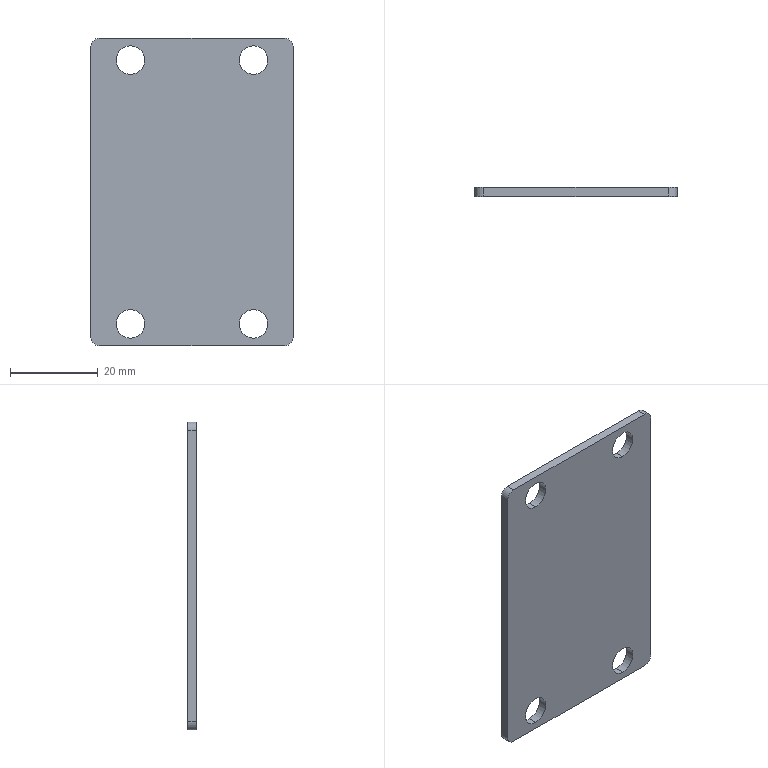Part | SolidWorks | features BaseBody 1 | 1 solid | 18 faces | box 46 x 2 x 70 mm | volume 6168 mm3 | cylinder 12 | plane 6 | commonest cylinder face diameters 6.5 x8 4 x4
STEP:
#1=CARTESIAN_POINT('',(-14.,0.,-26.75));
#2=VERTEX_POINT('',#1);
#3=CARTESIAN_POINT('',(-14.,0.,-33.25));
#4=VERTEX_POINT('',#3);
#5=CARTESIAN_POINT('',(-14.,0.,-30.));
#6=DIRECTION('',(0.,1.,0.));
#7=DIRECTION('',(0.,0.,1.));
#8=AXIS2_PLACEMENT_3D('',#5,#6,#7);
#9=CIRCLE('',#8,3.25);
#10=EDGE_CURVE('',#2,#4,#9,.T.);
#11=ORIENTED_EDGE('',*,*,#10,.T.);
#12=CARTESIAN_POINT('',(-14.,0.,-30.));
#13=DIRECTION('',(0.,1.,0.));
#14=DIRECTION('',(0.,0.,1.));
#15=AXIS2_PLACEMENT_3D('',#12,#13,#14);
#16=CIRCLE('',#15,3.25);
#17=EDGE_CURVE('',#4,#2,#16,.T.);
#18=ORIENTED_EDGE('',*,*,#17,.T.);
#19=EDGE_LOOP('',(#11,#18));
#20=FACE_BOUND('',#19,.T.);
#21=CARTESIAN_POINT('',(14.,0.,-26.75));
#22=VERTEX_POINT('',#21);
#23=CARTESIAN_POINT('',(14.,0.,-33.25));
#24=VERTEX_POINT('',#23);
#25=CARTESIAN_POINT('',(14.,0.,-30.));
#26=DIRECTION('',(0.,1.,0.));
#27=DIRECTION('',(0.,0.,1.));
#28=AXIS2_PLACEMENT_3D('',#25,#26,#27);
#29=CIRCLE('',#28,3.25);
#30=EDGE_CURVE('',#22,#24,#29,.T.);
#31=ORIENTED_EDGE('',*,*,#30,.T.);
#32=CARTESIAN_POINT('',(14.,0.,-30.));
#33=DIRECTION('',(0.,1.,0.));
#34=DIRECTION('',(0.,0.,1.));
#35=AXIS2_PLACEMENT_3D('',#32,#33,#34);
#36=CIRCLE('',#35,3.25);
#37=EDGE_CURVE('',#24,#22,#36,.T.);
#38=ORIENTED_EDGE('',*,*,#37,.T.);
#39=EDGE_LOOP('',(#31,#38));
#40=FACE_BOUND('',#39,.T.);
#41=CARTESIAN_POINT('',(-14.,0.,33.25));
#42=VERTEX_POINT('',#41);
#43=CARTESIAN_POINT('',(-14.,0.,26.75));
#44=VERTEX_POINT('',#43);
#45=CARTESIAN_POINT('',(-14.,0.,30.));
#46=DIRECTION('',(0.,1.,0.));
#47=DIRECTION('',(0.,0.,1.));
#48=AXIS2_PLACEMENT_3D('',#45,#46,#47);
#49=CIRCLE('',#48,3.25);
#50=EDGE_CURVE('',#42,#44,#49,.T.);
#51=ORIENTED_EDGE('',*,*,#50,.T.);
#52=CARTESIAN_POINT('',(-14.,0.,30.));
#53=DIRECTION('',(0.,1.,0.));
#54=DIRECTION('',(0.,0.,1.));
#55=AXIS2_PLACEMENT_3D('',#52,#53,#54);
#56=CIRCLE('',#55,3.25);
#57=EDGE_CURVE('',#44,#42,#56,.T.);
#58=ORIENTED_EDGE('',*,*,#57,.T.);
#59=EDGE_LOOP('',(#51,#58));
#60=FACE_BOUND('',#59,.T.);
#61=CARTESIAN_POINT('',(14.,0.,33.25));
#62=VERTEX_POINT('',#61);
#63=CARTESIAN_POINT('',(14.,0.,26.75));
#64=VERTEX_POINT('',#63);
#65=CARTESIAN_POINT('',(14.,0.,30.));
#66=DIRECTION('',(0.,1.,0.));
#67=DIRECTION('',(0.,0.,1.));
#68=AXIS2_PLACEMENT_3D('',#65,#66,#67);
#69=CIRCLE('',#68,3.25);
#70=EDGE_CURVE('',#62,#64,#69,.T.);
#71=ORIENTED_EDGE('',*,*,#70,.T.);
#72=CARTESIAN_POINT('',(14.,0.,30.));
#73=DIRECTION('',(0.,1.,0.));
#74=DIRECTION('',(0.,0.,1.));
#75=AXIS2_PLACEMENT_3D('',#72,#73,#74);
#76=CIRCLE('',#75,3.25);
#77=EDGE_CURVE('',#64,#62,#76,.T.);
#78=ORIENTED_EDGE('',*,*,#77,.T.);
#79=EDGE_LOOP('',(#71,#78));
#80=FACE_BOUND('',#79,.T.);
#81=CARTESIAN_POINT('',(-23.,0.,33.));
#82=VERTEX_POINT('',#81);
#83=CARTESIAN_POINT('',(-23.,0.,-33.));
#84=VERTEX_POINT('',#83);
#85=CARTESIAN_POINT('',(-23.,0.,-35.));
#86=DIRECTION('',(0.,0.,-1.));
#87=VECTOR('',#86,1000.);
#88=LINE('',#85,#87);
#89=EDGE_CURVE('',#82,#84,#88,.T.);
#90=ORIENTED_EDGE('',*,*,#89,.T.);
#91=CARTESIAN_POINT('',(-21.,0.,-35.));
#92=VERTEX_POINT('',#91);
#93=CARTESIAN_POINT('',(-21.,0.,-33.));
#94=DIRECTION('',(0.,1.,0.));
#95=DIRECTION('',(0.,0.,-1.));
#96=AXIS2_PLACEMENT_3D('',#93,#94,#95);
#97=CIRCLE('',#96,2.);
#98=EDGE_CURVE('',#92,#84,#97,.T.);
#99=ORIENTED_EDGE('',*,*,#98,.F.);
#100=CARTESIAN_POINT('',(21.,0.,-35.));
#101=VERTEX_POINT('',#100);
#102=CARTESIAN_POINT('',(-23.,0.,-35.));
#103=DIRECTION('',(1.,0.,0.));
#104=VECTOR('',#103,1000.);
#105=LINE('',#102,#104);
#106=EDGE_CURVE('',#92,#101,#105,.T.);
#107=ORIENTED_EDGE('',*,*,#106,.T.);
#108=CARTESIAN_POINT('',(23.,0.,-33.));
#109=VERTEX_POINT('',#108);
#110=CARTESIAN_POINT('',(21.,0.,-33.));
#111=DIRECTION('',(0.,1.,0.));
#112=DIRECTION('',(0.,0.,-1.));
#113=AXIS2_PLACEMENT_3D('',#110,#111,#112);
#114=CIRCLE('',#113,2.);
#115=EDGE_CURVE('',#109,#101,#114,.T.);
#116=ORIENTED_EDGE('',*,*,#115,.F.);
#117=CARTESIAN_POINT('',(23.,0.,33.));
#118=VERTEX_POINT('',#117);
#119=CARTESIAN_POINT('',(23.,0.,-35.));
#120=DIRECTION('',(0.,0.,1.));
#121=VECTOR('',#120,1000.);
#122=LINE('',#119,#121);
#123=EDGE_CURVE('',#109,#118,#122,.T.);
#124=ORIENTED_EDGE('',*,*,#123,.T.);
#125=CARTESIAN_POINT('',(21.,0.,35.));
#126=VERTEX_POINT('',#125);
#127=CARTESIAN_POINT('',(21.,0.,33.));
#128=DIRECTION('',(0.,1.,0.));
#129=DIRECTION('',(0.,0.,-1.));
#130=AXIS2_PLACEMENT_3D('',#127,#128,#129);
#131=CIRCLE('',#130,2.);
#132=EDGE_CURVE('',#126,#118,#131,.T.);
#133=ORIENTED_EDGE('',*,*,#132,.F.);
#134=CARTESIAN_POINT('',(-21.,0.,35.));
#135=VERTEX_POINT('',#134);
#136=CARTESIAN_POINT('',(-23.,0.,35.));
#137=DIRECTION('',(-1.,0.,0.));
#138=VECTOR('',#137,1000.);
#139=LINE('',#136,#138);
#140=EDGE_CURVE('',#126,#135,#139,.T.);
#141=ORIENTED_EDGE('',*,*,#140,.T.);
#142=CARTESIAN_POINT('',(-21.,0.,33.));
#143=DIRECTION('',(0.,1.,0.));
#144=DIRECTION('',(0.,0.,-1.));
#145=AXIS2_PLACEMENT_3D('',#142,#143,#144);
#146=CIRCLE('',#145,2.);
#147=EDGE_CURVE('',#82,#135,#146,.T.);
#148=ORIENTED_EDGE('',*,*,#147,.F.);
#149=EDGE_LOOP('',(#90,#99,#107,#116,#124,#133,#141,#148));
#150=FACE_OUTER_BOUND('',#149,.T.);
#151=CARTESIAN_POINT('',(0.,0.,0.));
#152=DIRECTION('',(0.,1.,0.));
#153=DIRECTION('',(1.,0.,0.));
#154=AXIS2_PLACEMENT_3D('',#151,#152,#153);
#155=PLANE('',#154);
#156=ADVANCED_FACE('',(#20,#40,#60,#80,#150),#155,.F.);
#157=ORIENTED_EDGE('',*,*,#106,.F.);
#158=CARTESIAN_POINT('',(-21.,2.,-35.));
#159=VERTEX_POINT('',#158);
#160=CARTESIAN_POINT('',(-21.,2.,-35.));
#161=DIRECTION('',(0.,-1.,0.));
#162=VECTOR('',#161,1000.);
#163=LINE('',#160,#162);
#164=EDGE_CURVE('',#159,#92,#163,.T.);
#165=ORIENTED_EDGE('',*,*,#164,.F.);
#166=CARTESIAN_POINT('',(21.,2.,-35.));
#167=VERTEX_POINT('',#166);
#168=CARTESIAN_POINT('',(0.,2.,-35.));
#169=DIRECTION('',(-1.,0.,0.));
#170=VECTOR('',#169,1000.);
#171=LINE('',#168,#170);
#172=EDGE_CURVE('',#167,#159,#171,.T.);
#173=ORIENTED_EDGE('',*,*,#172,.F.);
#174=CARTESIAN_POINT('',(21.,2.,-35.));
#175=DIRECTION('',(0.,1.,0.));
#176=VECTOR('',#175,1000.);
#177=LINE('',#174,#176);
#178=EDGE_CURVE('',#101,#167,#177,.T.);
#179=ORIENTED_EDGE('',*,*,#178,.F.);
#180=EDGE_LOOP('',(#157,#165,#173,#179));
#181=FACE_OUTER_BOUND('',#180,.T.);
#182=CARTESIAN_POINT('',(-23.,2.,-35.));
#183=DIRECTION('',(0.,0.,1.));
#184=DIRECTION('',(1.,0.,0.));
#185=AXIS2_PLACEMENT_3D('',#182,#183,#184);
#186=PLANE('',#185);
#187=ADVANCED_FACE('',(#181),#186,.F.);
#188=CARTESIAN_POINT('',(-23.,2.,-33.));
#189=VERTEX_POINT('',#188);
#190=CARTESIAN_POINT('',(-21.,2.,-33.));
#191=DIRECTION('',(0.,1.,0.));
#192=DIRECTION('',(0.,0.,-1.));
#193=AXIS2_PLACEMENT_3D('',#190,#191,#192);
#194=CIRCLE('',#193,2.);
#195=EDGE_CURVE('',#159,#189,#194,.T.);
#196=ORIENTED_EDGE('',*,*,#195,.F.);
#197=ORIENTED_EDGE('',*,*,#164,.T.);
#198=ORIENTED_EDGE('',*,*,#98,.T.);
#199=CARTESIAN_POINT('',(-23.,2.,-33.));
#200=DIRECTION('',(0.,1.,0.));
#201=VECTOR('',#200,1000.);
#202=LINE('',#199,#201);
#203=EDGE_CURVE('',#84,#189,#202,.T.);
#204=ORIENTED_EDGE('',*,*,#203,.T.);
#205=EDGE_LOOP('',(#196,#197,#198,#204));
#206=FACE_OUTER_BOUND('',#205,.T.);
#207=CARTESIAN_POINT('',(-21.,2.,-33.));
#208=DIRECTION('',(0.,-1.,0.));
#209=DIRECTION('',(0.,0.,-1.));
#210=AXIS2_PLACEMENT_3D('',#207,#208,#209);
#211=CYLINDRICAL_SURFACE('',#210,2.);
#212=ADVANCED_FACE('',(#206),#211,.T.);
#213=CARTESIAN_POINT('',(-23.,2.,33.));
#214=VERTEX_POINT('',#213);
#215=CARTESIAN_POINT('',(-23.,2.,0.));
#216=DIRECTION('',(0.,0.,1.));
#217=VECTOR('',#216,1000.);
#218=LINE('',#215,#217);
#219=EDGE_CURVE('',#189,#214,#218,.T.);
#220=ORIENTED_EDGE('',*,*,#219,.F.);
#221=ORIENTED_EDGE('',*,*,#203,.F.);
#222=ORIENTED_EDGE('',*,*,#89,.F.);
#223=CARTESIAN_POINT('',(-23.,2.,33.));
#224=DIRECTION('',(0.,-1.,0.));
#225=VECTOR('',#224,1000.);
#226=LINE('',#223,#225);
#227=EDGE_CURVE('',#214,#82,#226,.T.);
#228=ORIENTED_EDGE('',*,*,#227,.F.);
#229=EDGE_LOOP('',(#220,#221,#222,#228));
#230=FACE_OUTER_BOUND('',#229,.T.);
#231=CARTESIAN_POINT('',(-23.,2.,-35.));
#232=DIRECTION('',(1.,0.,0.));
#233=DIRECTION('',(0.,0.,-1.));
#234=AXIS2_PLACEMENT_3D('',#231,#232,#233);
#235=PLANE('',#234);
#236=ADVANCED_FACE('',(#230),#235,.F.);
#237=CARTESIAN_POINT('',(-21.,2.,35.));
#238=VERTEX_POINT('',#237);
#239=CARTESIAN_POINT('',(-21.,2.,33.));
#240=DIRECTION('',(0.,1.,0.));
#241=DIRECTION('',(0.,0.,-1.));
#242=AXIS2_PLACEMENT_3D('',#239,#240,#241);
#243=CIRCLE('',#242,2.);
#244=EDGE_CURVE('',#214,#238,#243,.T.);
#245=ORIENTED_EDGE('',*,*,#244,.F.);
#246=ORIENTED_EDGE('',*,*,#227,.T.);
#247=ORIENTED_EDGE('',*,*,#147,.T.);
#248=CARTESIAN_POINT('',(-21.,2.,35.));
#249=DIRECTION('',(0.,1.,0.));
#250=VECTOR('',#249,1000.);
#251=LINE('',#248,#250);
#252=EDGE_CURVE('',#135,#238,#251,.T.);
#253=ORIENTED_EDGE('',*,*,#252,.T.);
#254=EDGE_LOOP('',(#245,#246,#247,#253));
#255=FACE_OUTER_BOUND('',#254,.T.);
#256=CARTESIAN_POINT('',(-21.,2.,33.));
#257=DIRECTION('',(0.,-1.,0.));
#258=DIRECTION('',(0.,0.,-1.));
#259=AXIS2_PLACEMENT_3D('',#256,#257,#258);
#260=CYLINDRICAL_SURFACE('',#259,2.);
#261=ADVANCED_FACE('',(#255),#260,.T.);
#262=ORIENTED_EDGE('',*,*,#140,.F.);
#263=CARTESIAN_POINT('',(21.,2.,35.));
#264=VERTEX_POINT('',#263);
#265=CARTESIAN_POINT('',(21.,2.,35.));
#266=DIRECTION('',(0.,-1.,0.));
#267=VECTOR('',#266,1000.);
#268=LINE('',#265,#267);
#269=EDGE_CURVE('',#264,#126,#268,.T.);
#270=ORIENTED_EDGE('',*,*,#269,.F.);
#271=CARTESIAN_POINT('',(0.,2.,35.));
#272=DIRECTION('',(1.,0.,0.));
#273=VECTOR('',#272,1000.);
#274=LINE('',#271,#273);
#275=EDGE_CURVE('',#238,#264,#274,.T.);
#276=ORIENTED_EDGE('',*,*,#275,.F.);
#277=ORIENTED_EDGE('',*,*,#252,.F.);
#278=EDGE_LOOP('',(#262,#270,#276,#277));
#279=FACE_OUTER_BOUND('',#278,.T.);
#280=CARTESIAN_POINT('',(-23.,2.,35.));
#281=DIRECTION('',(0.,0.,-1.));
#282=DIRECTION('',(0.,-1.,0.));
#283=AXIS2_PLACEMENT_3D('',#280,#281,#282);
#284=PLANE('',#283);
#285=ADVANCED_FACE('',(#279),#284,.F.);
#286=CARTESIAN_POINT('',(23.,2.,33.));
#287=VERTEX_POINT('',#286);
#288=CARTESIAN_POINT('',(21.,2.,33.));
#289=DIRECTION('',(0.,1.,0.));
#290=DIRECTION('',(0.,0.,-1.));
#291=AXIS2_PLACEMENT_3D('',#288,#289,#290);
#292=CIRCLE('',#291,2.);
#293=EDGE_CURVE('',#264,#287,#292,.T.);
#294=ORIENTED_EDGE('',*,*,#293,.F.);
#295=ORIENTED_EDGE('',*,*,#269,.T.);
#296=ORIENTED_EDGE('',*,*,#132,.T.);
#297=CARTESIAN_POINT('',(23.,2.,33.));
#298=DIRECTION('',(0.,1.,0.));
#299=VECTOR('',#298,1000.);
#300=LINE('',#297,#299);
#301=EDGE_CURVE('',#118,#287,#300,.T.);
#302=ORIENTED_EDGE('',*,*,#301,.T.);
#303=EDGE_LOOP('',(#294,#295,#296,#302));
#304=FACE_OUTER_BOUND('',#303,.T.);
#305=CARTESIAN_POINT('',(21.,2.,33.));
#306=DIRECTION('',(0.,-1.,0.));
#307=DIRECTION('',(0.,0.,-1.));
#308=AXIS2_PLACEMENT_3D('',#305,#306,#307);
#309=CYLINDRICAL_SURFACE('',#308,2.);
#310=ADVANCED_FACE('',(#304),#309,.T.);
#311=ORIENTED_EDGE('',*,*,#123,.F.);
#312=CARTESIAN_POINT('',(23.,2.,-33.));
#313=VERTEX_POINT('',#312);
#314=CARTESIAN_POINT('',(23.,2.,-33.));
#315=DIRECTION('',(0.,-1.,0.));
#316=VECTOR('',#315,1000.);
#317=LINE('',#314,#316);
#318=EDGE_CURVE('',#313,#109,#317,.T.);
#319=ORIENTED_EDGE('',*,*,#318,.F.);
#320=CARTESIAN_POINT('',(23.,2.,0.));
#321=DIRECTION('',(0.,0.,-1.));
#322=VECTOR('',#321,1000.);
#323=LINE('',#320,#322);
#324=EDGE_CURVE('',#287,#313,#323,.T.);
#325=ORIENTED_EDGE('',*,*,#324,.F.);
#326=ORIENTED_EDGE('',*,*,#301,.F.);
#327=EDGE_LOOP('',(#311,#319,#325,#326));
#328=FACE_OUTER_BOUND('',#327,.T.);
#329=CARTESIAN_POINT('',(23.,2.,-35.));
#330=DIRECTION('',(-1.,0.,0.));
#331=DIRECTION('',(0.,1.,0.));
#332=AXIS2_PLACEMENT_3D('',#329,#330,#331);
#333=PLANE('',#332);
#334=ADVANCED_FACE('',(#328),#333,.F.);
#335=CARTESIAN_POINT('',(21.,2.,-33.));
#336=DIRECTION('',(0.,1.,0.));
#337=DIRECTION('',(0.,0.,-1.));
#338=AXIS2_PLACEMENT_3D('',#335,#336,#337);
#339=CIRCLE('',#338,2.);
#340=EDGE_CURVE('',#313,#167,#339,.T.);
#341=ORIENTED_EDGE('',*,*,#340,.F.);
#342=ORIENTED_EDGE('',*,*,#318,.T.);
#343=ORIENTED_EDGE('',*,*,#115,.T.);
#344=ORIENTED_EDGE('',*,*,#178,.T.);
#345=EDGE_LOOP('',(#341,#342,#343,#344));
#346=FACE_OUTER_BOUND('',#345,.T.);
#347=CARTESIAN_POINT('',(21.,2.,-33.));
#348=DIRECTION('',(0.,-1.,0.));
#349=DIRECTION('',(0.,0.,-1.));
#350=AXIS2_PLACEMENT_3D('',#347,#348,#349);
#351=CYLINDRICAL_SURFACE('',#350,2.);
#352=ADVANCED_FACE('',(#346),#351,.T.);
#353=CARTESIAN_POINT('',(-14.,2.,-33.25));
#354=VERTEX_POINT('',#353);
#355=CARTESIAN_POINT('',(-14.,2.,-33.25));
#356=DIRECTION('',(0.,1.,0.));
#357=VECTOR('',#356,1000.);
#358=LINE('',#355,#357);
#359=EDGE_CURVE('',#4,#354,#358,.T.);
#360=ORIENTED_EDGE('',*,*,#359,.F.);
#361=ORIENTED_EDGE('',*,*,#10,.F.);
#362=CARTESIAN_POINT('',(-14.,2.,-26.75));
#363=VERTEX_POINT('',#362);
#364=CARTESIAN_POINT('',(-14.,2.,-26.75));
#365=DIRECTION('',(0.,1.,0.));
#366=VECTOR('',#365,1000.);
#367=LINE('',#364,#366);
#368=EDGE_CURVE('',#2,#363,#367,.T.);
#369=ORIENTED_EDGE('',*,*,#368,.T.);
#370=CARTESIAN_POINT('',(-14.,2.,-30.));
#371=DIRECTION('',(0.,-1.,0.));
#372=DIRECTION('',(0.,0.,1.));
#373=AXIS2_PLACEMENT_3D('',#370,#371,#372);
#374=CIRCLE('',#373,3.25);
#375=EDGE_CURVE('',#354,#363,#374,.T.);
#376=ORIENTED_EDGE('',*,*,#375,.F.);
#377=EDGE_LOOP('',(#360,#361,#369,#376));
#378=FACE_OUTER_BOUND('',#377,.T.);
#379=CARTESIAN_POINT('',(-14.,2.,-30.));
#380=DIRECTION('',(0.,1.,0.));
#381=DIRECTION('',(0.,0.,1.));
#382=AXIS2_PLACEMENT_3D('',#379,#380,#381);
#383=CYLINDRICAL_SURFACE('',#382,3.25);
#384=ADVANCED_FACE('',(#378),#383,.F.);
#385=CARTESIAN_POINT('',(14.,2.,-33.25));
#386=VERTEX_POINT('',#385);
#387=CARTESIAN_POINT('',(14.,2.,-33.25));
#388=DIRECTION('',(0.,1.,0.));
#389=VECTOR('',#388,1000.);
#390=LINE('',#387,#389);
#391=EDGE_CURVE('',#24,#386,#390,.T.);
#392=ORIENTED_EDGE('',*,*,#391,.F.);
#393=ORIENTED_EDGE('',*,*,#30,.F.);
#394=CARTESIAN_POINT('',(14.,2.,-26.75));
#395=VERTEX_POINT('',#394);
#396=CARTESIAN_POINT('',(14.,2.,-26.75));
#397=DIRECTION('',(0.,1.,0.));
#398=VECTOR('',#397,1000.);
#399=LINE('',#396,#398);
#400=EDGE_CURVE('',#22,#395,#399,.T.);
#401=ORIENTED_EDGE('',*,*,#400,.T.);
#402=CARTESIAN_POINT('',(14.,2.,-30.));
#403=DIRECTION('',(0.,-1.,0.));
#404=DIRECTION('',(0.,0.,1.));
#405=AXIS2_PLACEMENT_3D('',#402,#403,#404);
#406=CIRCLE('',#405,3.25);
#407=EDGE_CURVE('',#386,#395,#406,.T.);
#408=ORIENTED_EDGE('',*,*,#407,.F.);
#409=EDGE_LOOP('',(#392,#393,#401,#408));
#410=FACE_OUTER_BOUND('',#409,.T.);
#411=CARTESIAN_POINT('',(14.,2.,-30.));
#412=DIRECTION('',(0.,1.,0.));
#413=DIRECTION('',(0.,0.,1.));
#414=AXIS2_PLACEMENT_3D('',#411,#412,#413);
#415=CYLINDRICAL_SURFACE('',#414,3.25);
#416=ADVANCED_FACE('',(#410),#415,.F.);
#417=CARTESIAN_POINT('',(-14.,2.,26.75));
#418=VERTEX_POINT('',#417);
#419=CARTESIAN_POINT('',(-14.,2.,26.75));
#420=DIRECTION('',(0.,1.,0.));
#421=VECTOR('',#420,1000.);
#422=LINE('',#419,#421);
#423=EDGE_CURVE('',#44,#418,#422,.T.);
#424=ORIENTED_EDGE('',*,*,#423,.F.);
#425=ORIENTED_EDGE('',*,*,#50,.F.);
#426=CARTESIAN_POINT('',(-14.,2.,33.25));
#427=VERTEX_POINT('',#426);
#428=CARTESIAN_POINT('',(-14.,2.,33.25));
#429=DIRECTION('',(0.,1.,0.));
#430=VECTOR('',#429,1000.);
#431=LINE('',#428,#430);
#432=EDGE_CURVE('',#42,#427,#431,.T.);
#433=ORIENTED_EDGE('',*,*,#432,.T.);
#434=CARTESIAN_POINT('',(-14.,2.,30.));
#435=DIRECTION('',(0.,-1.,0.));
#436=DIRECTION('',(0.,0.,1.));
#437=AXIS2_PLACEMENT_3D('',#434,#435,#436);
#438=CIRCLE('',#437,3.25);
#439=EDGE_CURVE('',#418,#427,#438,.T.);
#440=ORIENTED_EDGE('',*,*,#439,.F.);
#441=EDGE_LOOP('',(#424,#425,#433,#440));
#442=FACE_OUTER_BOUND('',#441,.T.);
#443=CARTESIAN_POINT('',(-14.,2.,30.));
#444=DIRECTION('',(0.,1.,0.));
#445=DIRECTION('',(0.,0.,1.));
#446=AXIS2_PLACEMENT_3D('',#443,#444,#445);
#447=CYLINDRICAL_SURFACE('',#446,3.25);
#448=ADVANCED_FACE('',(#442),#447,.F.);
#449=CARTESIAN_POINT('',(14.,2.,26.75));
#450=VERTEX_POINT('',#449);
#451=CARTESIAN_POINT('',(14.,2.,26.75));
#452=DIRECTION('',(0.,1.,0.));
#453=VECTOR('',#452,1000.);
#454=LINE('',#451,#453);
#455=EDGE_CURVE('',#64,#450,#454,.T.);
#456=ORIENTED_EDGE('',*,*,#455,.F.);
#457=ORIENTED_EDGE('',*,*,#70,.F.);
#458=CARTESIAN_POINT('',(14.,2.,33.25));
#459=VERTEX_POINT('',#458);
#460=CARTESIAN_POINT('',(14.,2.,33.25));
#461=DIRECTION('',(0.,1.,0.));
#462=VECTOR('',#461,1000.);
#463=LINE('',#460,#462);
#464=EDGE_CURVE('',#62,#459,#463,.T.);
#465=ORIENTED_EDGE('',*,*,#464,.T.);
#466=CARTESIAN_POINT('',(14.,2.,30.));
#467=DIRECTION('',(0.,-1.,0.));
#468=DIRECTION('',(0.,0.,1.));
#469=AXIS2_PLACEMENT_3D('',#466,#467,#468);
#470=CIRCLE('',#469,3.25);
#471=EDGE_CURVE('',#450,#459,#470,.T.);
#472=ORIENTED_EDGE('',*,*,#471,.F.);
#473=EDGE_LOOP('',(#456,#457,#465,#472));
#474=FACE_OUTER_BOUND('',#473,.T.);
#475=CARTESIAN_POINT('',(14.,2.,30.));
#476=DIRECTION('',(0.,1.,0.));
#477=DIRECTION('',(0.,0.,1.));
#478=AXIS2_PLACEMENT_3D('',#475,#476,#477);
#479=CYLINDRICAL_SURFACE('',#478,3.25);
#480=ADVANCED_FACE('',(#474),#479,.F.);
#481=CARTESIAN_POINT('',(-14.,2.,-30.));
#482=DIRECTION('',(0.,-1.,0.));
#483=DIRECTION('',(0.,0.,1.));
#484=AXIS2_PLACEMENT_3D('',#481,#482,#483);
#485=CIRCLE('',#484,3.25);
#486=EDGE_CURVE('',#363,#354,#485,.T.);
#487=ORIENTED_EDGE('',*,*,#486,.T.);
#488=ORIENTED_EDGE('',*,*,#375,.T.);
#489=EDGE_LOOP('',(#487,#488));
#490=FACE_BOUND('',#489,.T.);
#491=CARTESIAN_POINT('',(14.,2.,-30.));
#492=DIRECTION('',(0.,-1.,0.));
#493=DIRECTION('',(0.,0.,1.));
#494=AXIS2_PLACEMENT_3D('',#491,#492,#493);
#495=CIRCLE('',#494,3.25);
#496=EDGE_CURVE('',#395,#386,#495,.T.);
#497=ORIENTED_EDGE('',*,*,#496,.T.);
#498=ORIENTED_EDGE('',*,*,#407,.T.);
#499=EDGE_LOOP('',(#497,#498));
#500=FACE_BOUND('',#499,.T.);
#501=CARTESIAN_POINT('',(-14.,2.,30.));
#502=DIRECTION('',(0.,-1.,0.));
#503=DIRECTION('',(0.,0.,1.));
#504=AXIS2_PLACEMENT_3D('',#501,#502,#503);
#505=CIRCLE('',#504,3.25);
#506=EDGE_CURVE('',#427,#418,#505,.T.);
#507=ORIENTED_EDGE('',*,*,#506,.T.);
#508=ORIENTED_EDGE('',*,*,#439,.T.);
#509=EDGE_LOOP('',(#507,#508));
#510=FACE_BOUND('',#509,.T.);
#511=CARTESIAN_POINT('',(14.,2.,30.));
#512=DIRECTION('',(0.,-1.,0.));
#513=DIRECTION('',(0.,0.,1.));
#514=AXIS2_PLACEMENT_3D('',#511,#512,#513);
#515=CIRCLE('',#514,3.25);
#516=EDGE_CURVE('',#459,#450,#515,.T.);
#517=ORIENTED_EDGE('',*,*,#516,.T.);
#518=ORIENTED_EDGE('',*,*,#471,.T.);
#519=EDGE_LOOP('',(#517,#518));
#520=FACE_BOUND('',#519,.T.);
#521=ORIENTED_EDGE('',*,*,#324,.T.);
#522=ORIENTED_EDGE('',*,*,#340,.T.);
#523=ORIENTED_EDGE('',*,*,#172,.T.);
#524=ORIENTED_EDGE('',*,*,#195,.T.);
#525=ORIENTED_EDGE('',*,*,#219,.T.);
#526=ORIENTED_EDGE('',*,*,#244,.T.);
#527=ORIENTED_EDGE('',*,*,#275,.T.);
#528=ORIENTED_EDGE('',*,*,#293,.T.);
#529=EDGE_LOOP('',(#521,#522,#523,#524,#525,#526,#527,#528));
#530=FACE_OUTER_BOUND('',#529,.T.);
#531=CARTESIAN_POINT('',(0.,2.,0.));
#532=DIRECTION('',(0.,1.,0.));
#533=DIRECTION('',(1.,0.,0.));
#534=AXIS2_PLACEMENT_3D('',#531,#532,#533);
#535=PLANE('',#534);
#536=ADVANCED_FACE('',(#490,#500,#510,#520,#530),#535,.T.);
#537=ORIENTED_EDGE('',*,*,#17,.F.);
#538=ORIENTED_EDGE('',*,*,#359,.T.);
#539=ORIENTED_EDGE('',*,*,#486,.F.);
#540=ORIENTED_EDGE('',*,*,#368,.F.);
#541=EDGE_LOOP('',(#537,#538,#539,#540));
#542=FACE_OUTER_BOUND('',#541,.T.);
#543=CARTESIAN_POINT('',(-14.,2.,-30.));
#544=DIRECTION('',(0.,1.,0.));
#545=DIRECTION('',(0.,0.,1.));
#546=AXIS2_PLACEMENT_3D('',#543,#544,#545);
#547=CYLINDRICAL_SURFACE('',#546,3.25);
#548=ADVANCED_FACE('',(#542),#547,.F.);
#549=ORIENTED_EDGE('',*,*,#37,.F.);
#550=ORIENTED_EDGE('',*,*,#391,.T.);
#551=ORIENTED_EDGE('',*,*,#496,.F.);
#552=ORIENTED_EDGE('',*,*,#400,.F.);
#553=EDGE_LOOP('',(#549,#550,#551,#552));
#554=FACE_OUTER_BOUND('',#553,.T.);
#555=CARTESIAN_POINT('',(14.,2.,-30.));
#556=DIRECTION('',(0.,1.,0.));
#557=DIRECTION('',(0.,0.,1.));
#558=AXIS2_PLACEMENT_3D('',#555,#556,#557);
#559=CYLINDRICAL_SURFACE('',#558,3.25);
#560=ADVANCED_FACE('',(#554),#559,.F.);
#561=ORIENTED_EDGE('',*,*,#57,.F.);
#562=ORIENTED_EDGE('',*,*,#423,.T.);
#563=ORIENTED_EDGE('',*,*,#506,.F.);
#564=ORIENTED_EDGE('',*,*,#432,.F.);
#565=EDGE_LOOP('',(#561,#562,#563,#564));
#566=FACE_OUTER_BOUND('',#565,.T.);
#567=CARTESIAN_POINT('',(-14.,2.,30.));
#568=DIRECTION('',(0.,1.,0.));
#569=DIRECTION('',(0.,0.,1.));
#570=AXIS2_PLACEMENT_3D('',#567,#568,#569);
#571=CYLINDRICAL_SURFACE('',#570,3.25);
#572=ADVANCED_FACE('',(#566),#571,.F.);
#573=ORIENTED_EDGE('',*,*,#77,.F.);
#574=ORIENTED_EDGE('',*,*,#455,.T.);
#575=ORIENTED_EDGE('',*,*,#516,.F.);
#576=ORIENTED_EDGE('',*,*,#464,.F.);
#577=EDGE_LOOP('',(#573,#574,#575,#576));
#578=FACE_OUTER_BOUND('',#577,.T.);
#579=CARTESIAN_POINT('',(14.,2.,30.));
#580=DIRECTION('',(0.,1.,0.));
#581=DIRECTION('',(0.,0.,1.));
#582=AXIS2_PLACEMENT_3D('',#579,#580,#581);
#583=CYLINDRICAL_SURFACE('',#582,3.25);
#584=ADVANCED_FACE('',(#578),#583,.F.);
#585=CLOSED_SHELL('',(#156,#187,#212,#236,#261,#285,#310,#334,#352,#384,#416,#448,#480,#536,#548,#560,#572,#584));
#586=MANIFOLD_SOLID_BREP('',#585);
#587=CARTESIAN_POINT('',(0.,0.,0.));
#588=DIRECTION('',(0.,0.,1.));
#589=DIRECTION('',(1.,0.,0.));
#590=AXIS2_PLACEMENT_3D('',#587,#588,#589);
#591=(LENGTH_UNIT()NAMED_UNIT(*)SI_UNIT(.MILLI.,.METRE.));
#592=UNCERTAINTY_MEASURE_WITH_UNIT(LENGTH_MEASURE(0.00001),#591,'','');
#593=(NAMED_UNIT(*)PLANE_ANGLE_UNIT()SI_UNIT($,.RADIAN.));
#594=(NAMED_UNIT(*)SI_UNIT($,.STERADIAN.)SOLID_ANGLE_UNIT());
#595=(GEOMETRIC_REPRESENTATION_CONTEXT(3)GLOBAL_UNCERTAINTY_ASSIGNED_CONTEXT((#592))GLOBAL_UNIT_ASSIGNED_CONTEXT((#591,#593,#594))REPRESENTATION_CONTEXT('',''));
#596=ADVANCED_BREP_SHAPE_REPRESENTATION('',(#586,#590),#595);